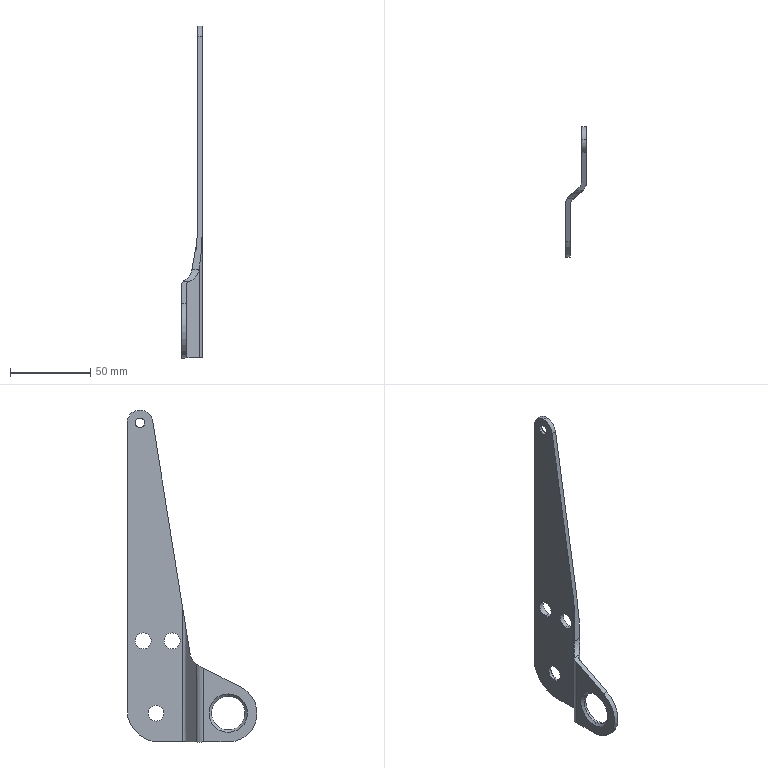Part | STEP file | 8XS174012 | 1 solid | 35 faces | box 13 x 81 x 207 mm | volume 21845 mm3 | cylinder 19 | plane 10 | cone 6 | commonest cylinder face diameters 10 x6 6 x4 12 x2 16 x2 21 x2 20 x1